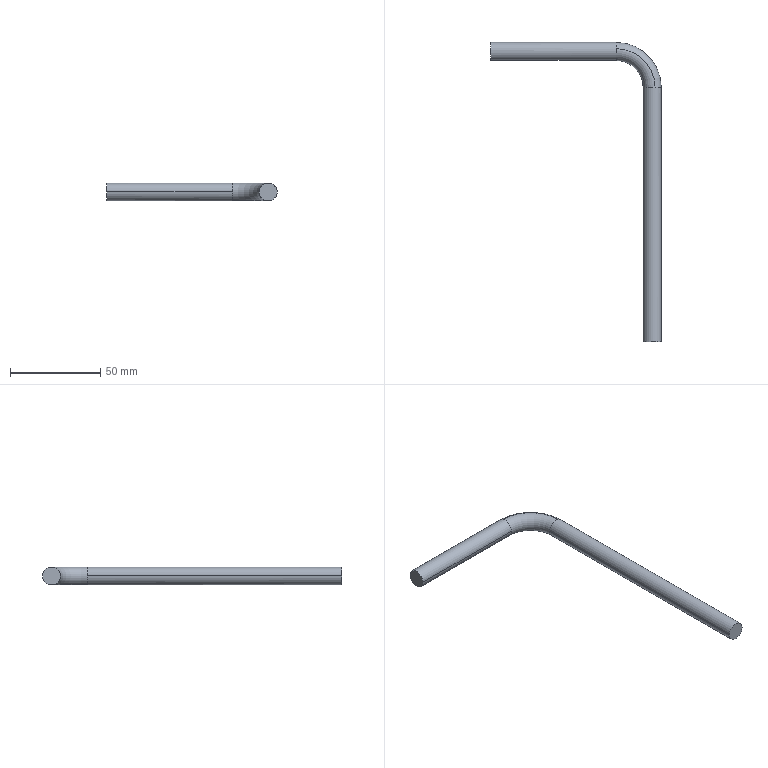Part | 1 solid | 8 faces | box 94.634 x 166.025 x 10 mm | volume 19013 mm3 | cylinder 4 | plane 2 | torus 2 | commonest cylinder face diameters 10 x4
STEP:
#1=CARTESIAN_POINT('',(0.,0.,0.));
#2=DIRECTION('',(0.,0.,1.));
#3=DIRECTION('',(1.,0.,0.));
#4=AXIS2_PLACEMENT_3D('',#1,#2,#3);
#5=CARTESIAN_POINT('',(-437.297,241.551,-281.55));
#6=VERTEX_POINT('',#5);
#7=CARTESIAN_POINT('',(-437.297,100.526,-281.55));
#8=VERTEX_POINT('',#7);
#9=CARTESIAN_POINT('',(-437.297,241.551,-281.55));
#10=DIRECTION('',(0.,-1.,0.));
#11=VECTOR('',#10,1.);
#12=LINE('',#9,#11);
#13=CARTESIAN_POINT('',(-432.297,241.551,-281.55));
#14=DIRECTION('',(0.,-1.,0.));
#15=DIRECTION('',(0.,0.,1.));
#16=AXIS2_PLACEMENT_3D('',#13,#14,#15);
#17=CYLINDRICAL_SURFACE('',#16,5.);
#18=CARTESIAN_POINT('',(1.571,0.));
#19=DIRECTION('',(0.,1.));
#20=VECTOR('',#19,1.);
#21=LINE('',#18,#20);
#22=(GEOMETRIC_REPRESENTATION_CONTEXT(2)PARAMETRIC_REPRESENTATION_CONTEXT()REPRESENTATION_CONTEXT('',''));
#23=DEFINITIONAL_REPRESENTATION('',(#21),#22);
#24=PCURVE('',#17,#23);
#25=CARTESIAN_POINT('',(-432.297,241.551,-281.55));
#26=DIRECTION('',(0.,-1.,0.));
#27=DIRECTION('',(0.,0.,-1.));
#28=AXIS2_PLACEMENT_3D('',#25,#26,#27);
#29=CYLINDRICAL_SURFACE('',#28,5.);
#30=CARTESIAN_POINT('',(4.712,0.));
#31=DIRECTION('',(0.,1.));
#32=VECTOR('',#31,1.);
#33=LINE('',#30,#32);
#34=(GEOMETRIC_REPRESENTATION_CONTEXT(2)PARAMETRIC_REPRESENTATION_CONTEXT()REPRESENTATION_CONTEXT('',''));
#35=DEFINITIONAL_REPRESENTATION('',(#33),#34);
#36=PCURVE('',#29,#35);
#37=SURFACE_CURVE('',#12,(#24,#36),.PCURVE_S1.);
#38=EDGE_CURVE('',#6,#8,#37,.T.);
#39=ORIENTED_EDGE('',*,*,#38,.F.);
#40=CARTESIAN_POINT('',(-433.842,241.551,-286.305));
#41=VERTEX_POINT('',#40);
#42=CARTESIAN_POINT('',(-432.297,241.551,-281.55));
#43=DIRECTION('',(0.,-1.,0.));
#44=DIRECTION('',(1.,0.,0.));
#45=AXIS2_PLACEMENT_3D('',#42,#43,#44);
#46=CIRCLE('',#45,5.);
#47=CARTESIAN_POINT('',(-1.571,0.));
#48=DIRECTION('',(1.,0.));
#49=VECTOR('',#48,1.);
#50=LINE('',#47,#49);
#51=(GEOMETRIC_REPRESENTATION_CONTEXT(2)PARAMETRIC_REPRESENTATION_CONTEXT()REPRESENTATION_CONTEXT('',''));
#52=DEFINITIONAL_REPRESENTATION('',(#50),#51);
#53=PCURVE('',#17,#52);
#54=CARTESIAN_POINT('',(-452.297,241.551,-281.55));
#55=DIRECTION('',(0.,0.,1.));
#56=DIRECTION('',(-0.7071,-0.7071,0.));
#57=AXIS2_PLACEMENT_3D('',#54,#55,#56);
#58=TOROIDAL_SURFACE('',#57,20.,5.);
#59=CARTESIAN_POINT('',(2.356,0.));
#60=DIRECTION('',(0.,1.));
#61=VECTOR('',#60,1.);
#62=LINE('',#59,#61);
#63=(GEOMETRIC_REPRESENTATION_CONTEXT(2)PARAMETRIC_REPRESENTATION_CONTEXT()REPRESENTATION_CONTEXT('',''));
#64=DEFINITIONAL_REPRESENTATION('',(#62),#63);
#65=PCURVE('',#58,#64);
#66=SURFACE_CURVE('',#46,(#53,#65),.PCURVE_S1.);
#67=EDGE_CURVE('',#6,#41,#66,.T.);
#68=ORIENTED_EDGE('',*,*,#67,.T.);
#69=CARTESIAN_POINT('',(-427.297,241.551,-281.55));
#70=VERTEX_POINT('',#69);
#71=CARTESIAN_POINT('',(-432.297,241.551,-281.55));
#72=DIRECTION('',(0.,-1.,0.));
#73=DIRECTION('',(1.,0.,0.));
#74=AXIS2_PLACEMENT_3D('',#71,#72,#73);
#75=CIRCLE('',#74,5.);
#76=CARTESIAN_POINT('',(-1.571,0.));
#77=DIRECTION('',(1.,0.));
#78=VECTOR('',#77,1.);
#79=LINE('',#76,#78);
#80=(GEOMETRIC_REPRESENTATION_CONTEXT(2)PARAMETRIC_REPRESENTATION_CONTEXT()REPRESENTATION_CONTEXT('',''));
#81=DEFINITIONAL_REPRESENTATION('',(#79),#80);
#82=PCURVE('',#17,#81);
#83=CARTESIAN_POINT('',(-452.297,241.551,-281.55));
#84=DIRECTION('',(0.,0.,1.));
#85=DIRECTION('',(-0.7071,-0.7071,0.));
#86=AXIS2_PLACEMENT_3D('',#83,#84,#85);
#87=TOROIDAL_SURFACE('',#86,20.,5.);
#88=CARTESIAN_POINT('',(2.356,0.));
#89=DIRECTION('',(0.,1.));
#90=VECTOR('',#89,1.);
#91=LINE('',#88,#90);
#92=(GEOMETRIC_REPRESENTATION_CONTEXT(2)PARAMETRIC_REPRESENTATION_CONTEXT()REPRESENTATION_CONTEXT('',''));
#93=DEFINITIONAL_REPRESENTATION('',(#91),#92);
#94=PCURVE('',#87,#93);
#95=SURFACE_CURVE('',#75,(#82,#94),.PCURVE_S1.);
#96=EDGE_CURVE('',#41,#70,#95,.T.);
#97=ORIENTED_EDGE('',*,*,#96,.T.);
#98=CARTESIAN_POINT('',(-427.297,100.526,-281.55));
#99=VERTEX_POINT('',#98);
#100=CARTESIAN_POINT('',(-427.297,241.551,-281.55));
#101=DIRECTION('',(0.,-1.,0.));
#102=VECTOR('',#101,1.);
#103=LINE('',#100,#102);
#104=CARTESIAN_POINT('',(4.712,0.));
#105=DIRECTION('',(0.,1.));
#106=VECTOR('',#105,1.);
#107=LINE('',#104,#106);
#108=(GEOMETRIC_REPRESENTATION_CONTEXT(2)PARAMETRIC_REPRESENTATION_CONTEXT()REPRESENTATION_CONTEXT('',''));
#109=DEFINITIONAL_REPRESENTATION('',(#107),#108);
#110=PCURVE('',#17,#109);
#111=CARTESIAN_POINT('',(1.571,0.));
#112=DIRECTION('',(0.,1.));
#113=VECTOR('',#112,1.);
#114=LINE('',#111,#113);
#115=(GEOMETRIC_REPRESENTATION_CONTEXT(2)PARAMETRIC_REPRESENTATION_CONTEXT()REPRESENTATION_CONTEXT('',''));
#116=DEFINITIONAL_REPRESENTATION('',(#114),#115);
#117=PCURVE('',#29,#116);
#118=SURFACE_CURVE('',#103,(#110,#117),.PCURVE_S1.);
#119=EDGE_CURVE('',#70,#99,#118,.T.);
#120=ORIENTED_EDGE('',*,*,#119,.T.);
#121=CARTESIAN_POINT('',(-432.297,100.526,-281.55));
#122=DIRECTION('',(0.,-1.,0.));
#123=DIRECTION('',(1.,0.,0.));
#124=AXIS2_PLACEMENT_3D('',#121,#122,#123);
#125=CIRCLE('',#124,5.);
#126=CARTESIAN_POINT('',(-1.571,141.025));
#127=DIRECTION('',(1.,0.));
#128=VECTOR('',#127,1.);
#129=LINE('',#126,#128);
#130=(GEOMETRIC_REPRESENTATION_CONTEXT(2)PARAMETRIC_REPRESENTATION_CONTEXT()REPRESENTATION_CONTEXT('',''));
#131=DEFINITIONAL_REPRESENTATION('',(#129),#130);
#132=PCURVE('',#17,#131);
#133=CARTESIAN_POINT('',(-402.025,100.526,-238.599));
#134=DIRECTION('',(0.,-1.,0.));
#135=DIRECTION('',(-1.,0.,0.));
#136=AXIS2_PLACEMENT_3D('',#133,#134,#135);
#137=PLANE('',#136);
#138=CARTESIAN_POINT('',(30.271,42.951));
#139=DIRECTION('',(-1.,0.));
#140=AXIS2_PLACEMENT_2D('',#138,#139);
#141=CIRCLE('',#140,5.);
#142=(GEOMETRIC_REPRESENTATION_CONTEXT(2)PARAMETRIC_REPRESENTATION_CONTEXT()REPRESENTATION_CONTEXT('',''));
#143=DEFINITIONAL_REPRESENTATION('',(#141),#142);
#144=PCURVE('',#137,#143);
#145=SURFACE_CURVE('',#125,(#132,#144),.PCURVE_S1.);
#146=EDGE_CURVE('',#8,#99,#145,.T.);
#147=ORIENTED_EDGE('',*,*,#146,.F.);
#148=EDGE_LOOP('',(#39,#68,#97,#120,#147));
#149=FACE_BOUND('',#148,.T.);
#150=ADVANCED_FACE('',(#149),#17,.T.);
#151=CARTESIAN_POINT('',(-432.297,100.526,-281.55));
#152=DIRECTION('',(0.,-1.,0.));
#153=DIRECTION('',(1.,0.,0.));
#154=AXIS2_PLACEMENT_3D('',#151,#152,#153);
#155=CIRCLE('',#154,5.);
#156=CARTESIAN_POINT('',(30.271,42.951));
#157=DIRECTION('',(-1.,0.));
#158=AXIS2_PLACEMENT_2D('',#156,#157);
#159=CIRCLE('',#158,5.);
#160=(GEOMETRIC_REPRESENTATION_CONTEXT(2)PARAMETRIC_REPRESENTATION_CONTEXT()REPRESENTATION_CONTEXT('',''));
#161=DEFINITIONAL_REPRESENTATION('',(#159),#160);
#162=PCURVE('',#137,#161);
#163=CARTESIAN_POINT('',(1.571,141.025));
#164=DIRECTION('',(1.,0.));
#165=VECTOR('',#164,1.);
#166=LINE('',#163,#165);
#167=(GEOMETRIC_REPRESENTATION_CONTEXT(2)PARAMETRIC_REPRESENTATION_CONTEXT()REPRESENTATION_CONTEXT('',''));
#168=DEFINITIONAL_REPRESENTATION('',(#166),#167);
#169=PCURVE('',#29,#168);
#170=SURFACE_CURVE('',#155,(#162,#169),.PCURVE_S1.);
#171=EDGE_CURVE('',#99,#8,#170,.T.);
#172=ORIENTED_EDGE('',*,*,#171,.T.);
#173=ORIENTED_EDGE('',*,*,#146,.T.);
#174=EDGE_LOOP('',(#172,#173));
#175=FACE_BOUND('',#174,.T.);
#176=ADVANCED_FACE('',(#175),#137,.T.);
#177=CARTESIAN_POINT('',(-452.297,260.006,-286.305));
#178=VERTEX_POINT('',#177);
#179=CARTESIAN_POINT('',(-452.297,241.551,-286.305));
#180=DIRECTION('',(0.,0.,1.));
#181=DIRECTION('',(1.,0.,0.));
#182=AXIS2_PLACEMENT_3D('',#179,#180,#181);
#183=CIRCLE('',#182,18.455);
#184=CARTESIAN_POINT('',(2.356,4.398));
#185=DIRECTION('',(1.,0.));
#186=VECTOR('',#185,1.);
#187=LINE('',#184,#186);
#188=(GEOMETRIC_REPRESENTATION_CONTEXT(2)PARAMETRIC_REPRESENTATION_CONTEXT()REPRESENTATION_CONTEXT('',''));
#189=DEFINITIONAL_REPRESENTATION('',(#187),#188);
#190=PCURVE('',#58,#189);
#191=CARTESIAN_POINT('',(2.356,4.398));
#192=DIRECTION('',(1.,0.));
#193=VECTOR('',#192,1.);
#194=LINE('',#191,#193);
#195=(GEOMETRIC_REPRESENTATION_CONTEXT(2)PARAMETRIC_REPRESENTATION_CONTEXT()REPRESENTATION_CONTEXT('',''));
#196=DEFINITIONAL_REPRESENTATION('',(#194),#195);
#197=PCURVE('',#87,#196);
#198=SURFACE_CURVE('',#183,(#190,#197),.PCURVE_S1.);
#199=EDGE_CURVE('',#41,#178,#198,.T.);
#200=ORIENTED_EDGE('',*,*,#199,.F.);
#201=ORIENTED_EDGE('',*,*,#67,.F.);
#202=CARTESIAN_POINT('',(-430.751,241.551,-276.795));
#203=VERTEX_POINT('',#202);
#204=CARTESIAN_POINT('',(-432.297,241.551,-281.55));
#205=DIRECTION('',(0.,-1.,0.));
#206=DIRECTION('',(1.,0.,0.));
#207=AXIS2_PLACEMENT_3D('',#204,#205,#206);
#208=CIRCLE('',#207,5.);
#209=CARTESIAN_POINT('',(2.356,0.));
#210=DIRECTION('',(0.,1.));
#211=VECTOR('',#210,1.);
#212=LINE('',#209,#211);
#213=(GEOMETRIC_REPRESENTATION_CONTEXT(2)PARAMETRIC_REPRESENTATION_CONTEXT()REPRESENTATION_CONTEXT('',''));
#214=DEFINITIONAL_REPRESENTATION('',(#212),#213);
#215=PCURVE('',#58,#214);
#216=CARTESIAN_POINT('',(1.571,0.));
#217=DIRECTION('',(1.,0.));
#218=VECTOR('',#217,1.);
#219=LINE('',#216,#218);
#220=(GEOMETRIC_REPRESENTATION_CONTEXT(2)PARAMETRIC_REPRESENTATION_CONTEXT()REPRESENTATION_CONTEXT('',''));
#221=DEFINITIONAL_REPRESENTATION('',(#219),#220);
#222=PCURVE('',#29,#221);
#223=SURFACE_CURVE('',#208,(#215,#222),.PCURVE_S1.);
#224=EDGE_CURVE('',#203,#6,#223,.T.);
#225=ORIENTED_EDGE('',*,*,#224,.F.);
#226=CARTESIAN_POINT('',(-452.297,263.096,-276.795));
#227=VERTEX_POINT('',#226);
#228=CARTESIAN_POINT('',(-452.297,241.551,-276.795));
#229=DIRECTION('',(0.,0.,1.));
#230=DIRECTION('',(1.,0.,0.));
#231=AXIS2_PLACEMENT_3D('',#228,#229,#230);
#232=CIRCLE('',#231,21.545);
#233=CARTESIAN_POINT('',(2.356,1.257));
#234=DIRECTION('',(1.,0.));
#235=VECTOR('',#234,1.);
#236=LINE('',#233,#235);
#237=(GEOMETRIC_REPRESENTATION_CONTEXT(2)PARAMETRIC_REPRESENTATION_CONTEXT()REPRESENTATION_CONTEXT('',''));
#238=DEFINITIONAL_REPRESENTATION('',(#236),#237);
#239=PCURVE('',#58,#238);
#240=CARTESIAN_POINT('',(2.356,7.54));
#241=DIRECTION('',(1.,0.));
#242=VECTOR('',#241,1.);
#243=LINE('',#240,#242);
#244=(GEOMETRIC_REPRESENTATION_CONTEXT(2)PARAMETRIC_REPRESENTATION_CONTEXT()REPRESENTATION_CONTEXT('',''));
#245=DEFINITIONAL_REPRESENTATION('',(#243),#244);
#246=PCURVE('',#87,#245);
#247=SURFACE_CURVE('',#232,(#239,#246),.PCURVE_S1.);
#248=EDGE_CURVE('',#203,#227,#247,.T.);
#249=ORIENTED_EDGE('',*,*,#248,.T.);
#250=CARTESIAN_POINT('',(-452.297,256.551,-281.55));
#251=VERTEX_POINT('',#250);
#252=CARTESIAN_POINT('',(-452.297,261.551,-281.55));
#253=DIRECTION('',(1.,0.,0.));
#254=DIRECTION('',(0.,1.,0.));
#255=AXIS2_PLACEMENT_3D('',#252,#253,#254);
#256=CIRCLE('',#255,5.);
#257=CARTESIAN_POINT('',(3.927,0.));
#258=DIRECTION('',(0.,1.));
#259=VECTOR('',#258,1.);
#260=LINE('',#257,#259);
#261=(GEOMETRIC_REPRESENTATION_CONTEXT(2)PARAMETRIC_REPRESENTATION_CONTEXT()REPRESENTATION_CONTEXT('',''));
#262=DEFINITIONAL_REPRESENTATION('',(#260),#261);
#263=PCURVE('',#58,#262);
#264=CARTESIAN_POINT('',(-452.297,261.551,-281.55));
#265=DIRECTION('',(-1.,0.,0.));
#266=DIRECTION('',(0.,0.,-1.));
#267=AXIS2_PLACEMENT_3D('',#264,#265,#266);
#268=CYLINDRICAL_SURFACE('',#267,5.);
#269=CARTESIAN_POINT('',(4.712,0.));
#270=DIRECTION('',(-1.,0.));
#271=VECTOR('',#270,1.);
#272=LINE('',#269,#271);
#273=(GEOMETRIC_REPRESENTATION_CONTEXT(2)PARAMETRIC_REPRESENTATION_CONTEXT()REPRESENTATION_CONTEXT('',''));
#274=DEFINITIONAL_REPRESENTATION('',(#272),#273);
#275=PCURVE('',#268,#274);
#276=SURFACE_CURVE('',#256,(#263,#275),.PCURVE_S1.);
#277=EDGE_CURVE('',#227,#251,#276,.T.);
#278=ORIENTED_EDGE('',*,*,#277,.T.);
#279=CARTESIAN_POINT('',(-452.297,261.551,-281.55));
#280=DIRECTION('',(1.,0.,0.));
#281=DIRECTION('',(0.,1.,0.));
#282=AXIS2_PLACEMENT_3D('',#279,#280,#281);
#283=CIRCLE('',#282,5.);
#284=CARTESIAN_POINT('',(3.927,0.));
#285=DIRECTION('',(0.,1.));
#286=VECTOR('',#285,1.);
#287=LINE('',#284,#286);
#288=(GEOMETRIC_REPRESENTATION_CONTEXT(2)PARAMETRIC_REPRESENTATION_CONTEXT()REPRESENTATION_CONTEXT('',''));
#289=DEFINITIONAL_REPRESENTATION('',(#287),#288);
#290=PCURVE('',#58,#289);
#291=CARTESIAN_POINT('',(-452.297,261.551,-281.55));
#292=DIRECTION('',(-1.,0.,0.));
#293=DIRECTION('',(0.,0.,1.));
#294=AXIS2_PLACEMENT_3D('',#291,#292,#293);
#295=CYLINDRICAL_SURFACE('',#294,5.);
#296=CARTESIAN_POINT('',(7.854,0.));
#297=DIRECTION('',(-1.,0.));
#298=VECTOR('',#297,1.);
#299=LINE('',#296,#298);
#300=(GEOMETRIC_REPRESENTATION_CONTEXT(2)PARAMETRIC_REPRESENTATION_CONTEXT()REPRESENTATION_CONTEXT('',''));
#301=DEFINITIONAL_REPRESENTATION('',(#299),#300);
#302=PCURVE('',#295,#301);
#303=SURFACE_CURVE('',#283,(#290,#302),.PCURVE_S1.);
#304=EDGE_CURVE('',#251,#178,#303,.T.);
#305=ORIENTED_EDGE('',*,*,#304,.T.);
#306=EDGE_LOOP('',(#200,#201,#225,#249,#278,#305));
#307=FACE_BOUND('',#306,.T.);
#308=ADVANCED_FACE('',(#307),#58,.T.);
#309=CARTESIAN_POINT('',(-452.297,266.551,-281.55));
#310=VERTEX_POINT('',#309);
#311=CARTESIAN_POINT('',(-521.931,266.551,-281.55));
#312=VERTEX_POINT('',#311);
#313=CARTESIAN_POINT('',(-452.297,266.551,-281.55));
#314=DIRECTION('',(-1.,0.,0.));
#315=VECTOR('',#314,1.);
#316=LINE('',#313,#315);
#317=CARTESIAN_POINT('',(1.571,0.));
#318=DIRECTION('',(0.,1.));
#319=VECTOR('',#318,1.);
#320=LINE('',#317,#319);
#321=(GEOMETRIC_REPRESENTATION_CONTEXT(2)PARAMETRIC_REPRESENTATION_CONTEXT()REPRESENTATION_CONTEXT('',''));
#322=DEFINITIONAL_REPRESENTATION('',(#320),#321);
#323=PCURVE('',#295,#322);
#324=CARTESIAN_POINT('',(4.712,0.));
#325=DIRECTION('',(0.,1.));
#326=VECTOR('',#325,1.);
#327=LINE('',#324,#326);
#328=(GEOMETRIC_REPRESENTATION_CONTEXT(2)PARAMETRIC_REPRESENTATION_CONTEXT()REPRESENTATION_CONTEXT('',''));
#329=DEFINITIONAL_REPRESENTATION('',(#327),#328);
#330=PCURVE('',#268,#329);
#331=SURFACE_CURVE('',#316,(#323,#330),.PCURVE_S1.);
#332=EDGE_CURVE('',#310,#312,#331,.T.);
#333=ORIENTED_EDGE('',*,*,#332,.F.);
#334=CARTESIAN_POINT('',(-452.297,261.551,-281.55));
#335=DIRECTION('',(1.,0.,0.));
#336=DIRECTION('',(0.,1.,0.));
#337=AXIS2_PLACEMENT_3D('',#334,#335,#336);
#338=CIRCLE('',#337,5.);
#339=CARTESIAN_POINT('',(7.854,0.));
#340=DIRECTION('',(-1.,0.));
#341=VECTOR('',#340,1.);
#342=LINE('',#339,#341);
#343=(GEOMETRIC_REPRESENTATION_CONTEXT(2)PARAMETRIC_REPRESENTATION_CONTEXT()REPRESENTATION_CONTEXT('',''));
#344=DEFINITIONAL_REPRESENTATION('',(#342),#343);
#345=PCURVE('',#295,#344);
#346=CARTESIAN_POINT('',(3.927,0.));
#347=DIRECTION('',(0.,1.));
#348=VECTOR('',#347,1.);
#349=LINE('',#346,#348);
#350=(GEOMETRIC_REPRESENTATION_CONTEXT(2)PARAMETRIC_REPRESENTATION_CONTEXT()REPRESENTATION_CONTEXT('',''));
#351=DEFINITIONAL_REPRESENTATION('',(#349),#350);
#352=PCURVE('',#87,#351);
#353=SURFACE_CURVE('',#338,(#345,#352),.PCURVE_S1.);
#354=EDGE_CURVE('',#178,#310,#353,.T.);
#355=ORIENTED_EDGE('',*,*,#354,.F.);
#356=ORIENTED_EDGE('',*,*,#304,.F.);
#357=CARTESIAN_POINT('',(-521.931,256.551,-281.55));
#358=VERTEX_POINT('',#357);
#359=CARTESIAN_POINT('',(-452.297,256.551,-281.55));
#360=DIRECTION('',(-1.,0.,0.));
#361=VECTOR('',#360,1.);
#362=LINE('',#359,#361);
#363=CARTESIAN_POINT('',(4.712,0.));
#364=DIRECTION('',(0.,1.));
#365=VECTOR('',#364,1.);
#366=LINE('',#363,#365);
#367=(GEOMETRIC_REPRESENTATION_CONTEXT(2)PARAMETRIC_REPRESENTATION_CONTEXT()REPRESENTATION_CONTEXT('',''));
#368=DEFINITIONAL_REPRESENTATION('',(#366),#367);
#369=PCURVE('',#295,#368);
#370=CARTESIAN_POINT('',(1.571,0.));
#371=DIRECTION('',(0.,1.));
#372=VECTOR('',#371,1.);
#373=LINE('',#370,#372);
#374=(GEOMETRIC_REPRESENTATION_CONTEXT(2)PARAMETRIC_REPRESENTATION_CONTEXT()REPRESENTATION_CONTEXT('',''));
#375=DEFINITIONAL_REPRESENTATION('',(#373),#374);
#376=PCURVE('',#268,#375);
#377=SURFACE_CURVE('',#362,(#369,#376),.PCURVE_S1.);
#378=EDGE_CURVE('',#251,#358,#377,.T.);
#379=ORIENTED_EDGE('',*,*,#378,.T.);
#380=CARTESIAN_POINT('',(-521.931,261.551,-281.55));
#381=DIRECTION('',(1.,0.,0.));
#382=DIRECTION('',(0.,-1.,0.));
#383=AXIS2_PLACEMENT_3D('',#380,#381,#382);
#384=CIRCLE('',#383,5.);
#385=CARTESIAN_POINT('',(4.712,69.634));
#386=DIRECTION('',(-1.,0.));
#387=VECTOR('',#386,1.);
#388=LINE('',#385,#387);
#389=(GEOMETRIC_REPRESENTATION_CONTEXT(2)PARAMETRIC_REPRESENTATION_CONTEXT()REPRESENTATION_CONTEXT('',''));
#390=DEFINITIONAL_REPRESENTATION('',(#388),#389);
#391=PCURVE('',#295,#390);
#392=CARTESIAN_POINT('',(-521.931,261.551,-281.55));
#393=DIRECTION('',(1.,0.,0.));
#394=DIRECTION('',(0.,1.,0.));
#395=AXIS2_PLACEMENT_3D('',#392,#393,#394);
#396=PLANE('',#395);
#397=CARTESIAN_POINT('',(0.,0.));
#398=DIRECTION('',(-1.,0.));
#399=AXIS2_PLACEMENT_2D('',#397,#398);
#400=CIRCLE('',#399,5.);
#401=(GEOMETRIC_REPRESENTATION_CONTEXT(2)PARAMETRIC_REPRESENTATION_CONTEXT()REPRESENTATION_CONTEXT('',''));
#402=DEFINITIONAL_REPRESENTATION('',(#400),#401);
#403=PCURVE('',#396,#402);
#404=SURFACE_CURVE('',#384,(#391,#403),.PCURVE_S1.);
#405=EDGE_CURVE('',#358,#312,#404,.T.);
#406=ORIENTED_EDGE('',*,*,#405,.T.);
#407=EDGE_LOOP('',(#333,#355,#356,#379,#406));
#408=FACE_BOUND('',#407,.T.);
#409=ADVANCED_FACE('',(#408),#295,.T.);
#410=CARTESIAN_POINT('',(-521.931,261.551,-281.55));
#411=DIRECTION('',(1.,0.,0.));
#412=DIRECTION('',(0.,-1.,0.));
#413=AXIS2_PLACEMENT_3D('',#410,#411,#412);
#414=CIRCLE('',#413,5.);
#415=CARTESIAN_POINT('',(0.,0.));
#416=DIRECTION('',(-1.,0.));
#417=AXIS2_PLACEMENT_2D('',#415,#416);
#418=CIRCLE('',#417,5.);
#419=(GEOMETRIC_REPRESENTATION_CONTEXT(2)PARAMETRIC_REPRESENTATION_CONTEXT()REPRESENTATION_CONTEXT('',''));
#420=DEFINITIONAL_REPRESENTATION('',(#418),#419);
#421=PCURVE('',#396,#420);
#422=CARTESIAN_POINT('',(7.854,69.634));
#423=DIRECTION('',(-1.,0.));
#424=VECTOR('',#423,1.);
#425=LINE('',#422,#424);
#426=(GEOMETRIC_REPRESENTATION_CONTEXT(2)PARAMETRIC_REPRESENTATION_CONTEXT()REPRESENTATION_CONTEXT('',''));
#427=DEFINITIONAL_REPRESENTATION('',(#425),#426);
#428=PCURVE('',#268,#427);
#429=SURFACE_CURVE('',#414,(#421,#428),.PCURVE_S1.);
#430=EDGE_CURVE('',#312,#358,#429,.T.);
#431=ORIENTED_EDGE('',*,*,#430,.F.);
#432=ORIENTED_EDGE('',*,*,#405,.F.);
#433=EDGE_LOOP('',(#431,#432));
#434=FACE_BOUND('',#433,.T.);
#435=ADVANCED_FACE('',(#434),#396,.F.);
#436=ORIENTED_EDGE('',*,*,#38,.T.);
#437=ORIENTED_EDGE('',*,*,#171,.F.);
#438=ORIENTED_EDGE('',*,*,#119,.F.);
#439=CARTESIAN_POINT('',(-432.297,241.551,-281.55));
#440=DIRECTION('',(0.,-1.,0.));
#441=DIRECTION('',(1.,0.,0.));
#442=AXIS2_PLACEMENT_3D('',#439,#440,#441);
#443=CIRCLE('',#442,5.);
#444=CARTESIAN_POINT('',(1.571,0.));
#445=DIRECTION('',(1.,0.));
#446=VECTOR('',#445,1.);
#447=LINE('',#444,#446);
#448=(GEOMETRIC_REPRESENTATION_CONTEXT(2)PARAMETRIC_REPRESENTATION_CONTEXT()REPRESENTATION_CONTEXT('',''));
#449=DEFINITIONAL_REPRESENTATION('',(#447),#448);
#450=PCURVE('',#29,#449);
#451=CARTESIAN_POINT('',(2.356,6.283));
#452=DIRECTION('',(0.,1.));
#453=VECTOR('',#452,1.);
#454=LINE('',#451,#453);
#455=(GEOMETRIC_REPRESENTATION_CONTEXT(2)PARAMETRIC_REPRESENTATION_CONTEXT()REPRESENTATION_CONTEXT('',''));
#456=DEFINITIONAL_REPRESENTATION('',(#454),#455);
#457=PCURVE('',#87,#456);
#458=SURFACE_CURVE('',#443,(#450,#457),.PCURVE_S1.);
#459=EDGE_CURVE('',#70,#203,#458,.T.);
#460=ORIENTED_EDGE('',*,*,#459,.T.);
#461=ORIENTED_EDGE('',*,*,#224,.T.);
#462=EDGE_LOOP('',(#436,#437,#438,#460,#461));
#463=FACE_BOUND('',#462,.T.);
#464=ADVANCED_FACE('',(#463),#29,.T.);
#465=ORIENTED_EDGE('',*,*,#199,.T.);
#466=ORIENTED_EDGE('',*,*,#354,.T.);
#467=CARTESIAN_POINT('',(-452.297,261.551,-281.55));
#468=DIRECTION('',(1.,0.,0.));
#469=DIRECTION('',(0.,1.,0.));
#470=AXIS2_PLACEMENT_3D('',#467,#468,#469);
#471=CIRCLE('',#470,5.);
#472=CARTESIAN_POINT('',(3.927,6.283));
#473=DIRECTION('',(0.,1.));
#474=VECTOR('',#473,1.);
#475=LINE('',#472,#474);
#476=(GEOMETRIC_REPRESENTATION_CONTEXT(2)PARAMETRIC_REPRESENTATION_CONTEXT()REPRESENTATION_CONTEXT('',''));
#477=DEFINITIONAL_REPRESENTATION('',(#475),#476);
#478=PCURVE('',#87,#477);
#479=CARTESIAN_POINT('',(4.712,0.));
#480=DIRECTION('',(-1.,0.));
#481=VECTOR('',#480,1.);
#482=LINE('',#479,#481);
#483=(GEOMETRIC_REPRESENTATION_CONTEXT(2)PARAMETRIC_REPRESENTATION_CONTEXT()REPRESENTATION_CONTEXT('',''));
#484=DEFINITIONAL_REPRESENTATION('',(#482),#483);
#485=PCURVE('',#268,#484);
#486=SURFACE_CURVE('',#471,(#478,#485),.PCURVE_S1.);
#487=EDGE_CURVE('',#310,#227,#486,.T.);
#488=ORIENTED_EDGE('',*,*,#487,.T.);
#489=ORIENTED_EDGE('',*,*,#248,.F.);
#490=ORIENTED_EDGE('',*,*,#459,.F.);
#491=ORIENTED_EDGE('',*,*,#96,.F.);
#492=EDGE_LOOP('',(#465,#466,#488,#489,#490,#491));
#493=FACE_BOUND('',#492,.T.);
#494=ADVANCED_FACE('',(#493),#87,.T.);
#495=ORIENTED_EDGE('',*,*,#332,.T.);
#496=ORIENTED_EDGE('',*,*,#430,.T.);
#497=ORIENTED_EDGE('',*,*,#378,.F.);
#498=ORIENTED_EDGE('',*,*,#277,.F.);
#499=ORIENTED_EDGE('',*,*,#487,.F.);
#500=EDGE_LOOP('',(#495,#496,#497,#498,#499));
#501=FACE_BOUND('',#500,.T.);
#502=ADVANCED_FACE('',(#501),#268,.T.);
#503=CLOSED_SHELL('',(#150,#176,#308,#409,#435,#464,#494,#502));
#504=MANIFOLD_SOLID_BREP('',#503);
#505=(LENGTH_UNIT()NAMED_UNIT(*)SI_UNIT(.MILLI.,.METRE.));
#506=UNCERTAINTY_MEASURE_WITH_UNIT(LENGTH_MEASURE(0.0000001),#505,'','');
#507=(NAMED_UNIT(*)PLANE_ANGLE_UNIT()SI_UNIT($,.RADIAN.));
#508=(NAMED_UNIT(*)SI_UNIT($,.STERADIAN.)SOLID_ANGLE_UNIT());
#509=(GEOMETRIC_REPRESENTATION_CONTEXT(3)GLOBAL_UNCERTAINTY_ASSIGNED_CONTEXT((#506))GLOBAL_UNIT_ASSIGNED_CONTEXT((#505,#507,#508))REPRESENTATION_CONTEXT('',''));
#510=ADVANCED_BREP_SHAPE_REPRESENTATION('',(#4,#504),#509);